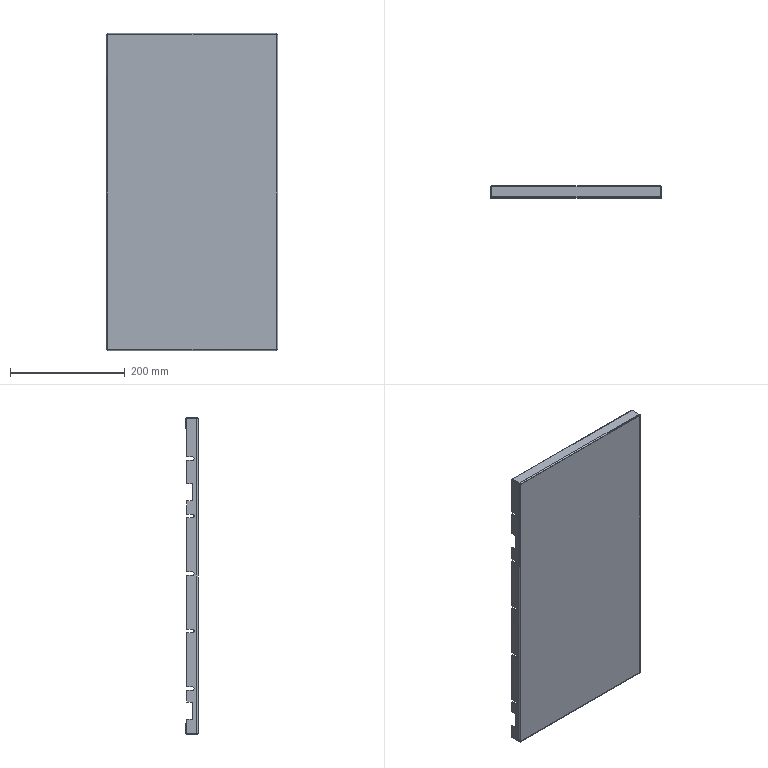Part | SolidWorks | features EdgeFlange 2, Cut 1, FlatPattern 1, HoleWzd 1, SMBaseFlange 1, SheetMetal 1 | 1 solid | 110 faces | box 298 x 21.5 x 551.5 mm | volume 305724 mm3 | plane 80 | cylinder 22 | spline 8 | commonest cylinder face diameters 5.8 x10 1.473 x6 4.473 x6